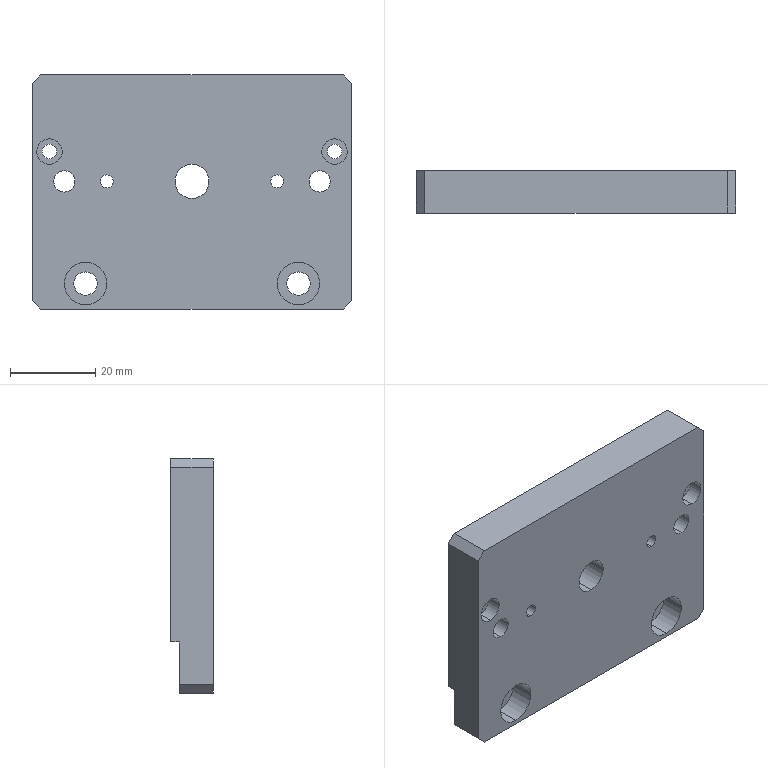Part | STEP file | PN_0033 | 1 solid | 42 faces | box 75 x 10 x 55 mm | volume 37025 mm3 | cylinder 26 | plane 16 | commonest cylinder face diameters 3 x4 3.4 x4 5 x4 5.5 x4 6 x4 10 x4